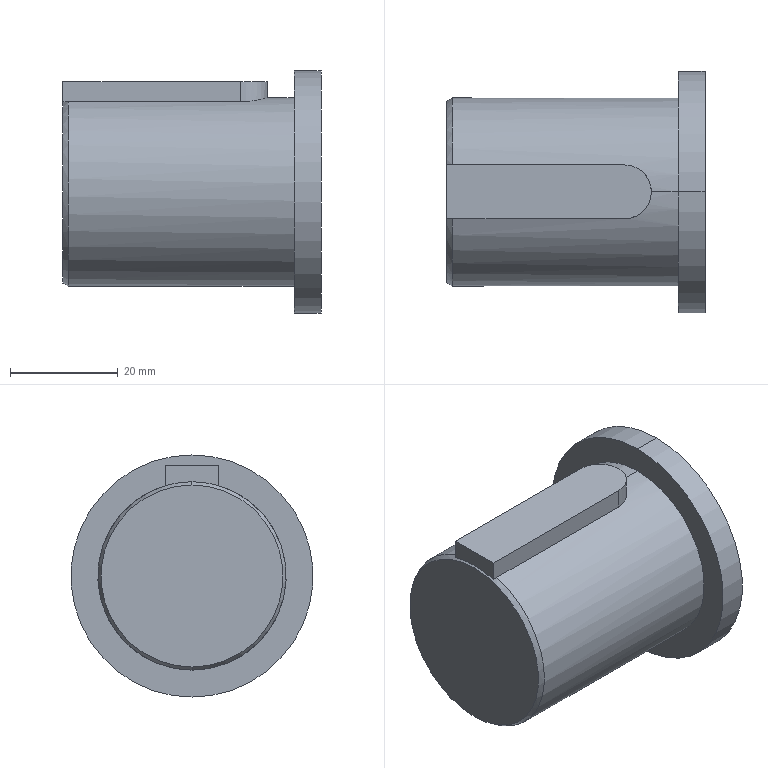Part | STEP file | 1 solid | 17 faces | box 48 x 45 x 45 mm | volume 50486 mm3 | cylinder 8 | plane 7 | cone 2 | commonest cylinder face diameters 35 x4 10 x2 45 x2
STEP:
#1=CARTESIAN_POINT('',(0.,0.,0.));
#2=DIRECTION('',(0.,0.,1.));
#3=DIRECTION('',(1.,0.,0.));
#4=AXIS2_PLACEMENT_3D('',#1,#2,#3);
#5=CARTESIAN_POINT('',(-134.,0.,-16.923));
#6=VERTEX_POINT('',#5);
#7=CARTESIAN_POINT('',(-133.,0.,-17.5));
#8=VERTEX_POINT('',#7);
#9=CARTESIAN_POINT('',(-133.5,0.,-17.211));
#10=DIRECTION('',(0.866,0.,-0.5));
#11=VECTOR('',#10,1.);
#12=LINE('',#9,#11);
#13=CARTESIAN_POINT('',(-133.5,0.,0.));
#14=DIRECTION('',(1.,0.,0.));
#15=DIRECTION('',(0.,0.,-1.));
#16=AXIS2_PLACEMENT_3D('',#13,#14,#15);
#17=CONICAL_SURFACE('',#16,17.211,0.5236);
#18=CARTESIAN_POINT('',(0.,0.));
#19=DIRECTION('',(0.,1.));
#20=VECTOR('',#19,1.);
#21=LINE('',#18,#20);
#22=(GEOMETRIC_REPRESENTATION_CONTEXT(2)PARAMETRIC_REPRESENTATION_CONTEXT()REPRESENTATION_CONTEXT('',''));
#23=DEFINITIONAL_REPRESENTATION('',(#21),#22);
#24=PCURVE('',#17,#23);
#25=CARTESIAN_POINT('',(-133.5,0.,0.));
#26=DIRECTION('',(1.,0.,0.));
#27=DIRECTION('',(0.,0.,-1.));
#28=AXIS2_PLACEMENT_3D('',#25,#26,#27);
#29=CONICAL_SURFACE('',#28,17.211,0.5236);
#30=CARTESIAN_POINT('',(6.283,0.));
#31=DIRECTION('',(0.,1.));
#32=VECTOR('',#31,1.);
#33=LINE('',#30,#32);
#34=(GEOMETRIC_REPRESENTATION_CONTEXT(2)PARAMETRIC_REPRESENTATION_CONTEXT()REPRESENTATION_CONTEXT('',''));
#35=DEFINITIONAL_REPRESENTATION('',(#33),#34);
#36=PCURVE('',#29,#35);
#37=SURFACE_CURVE('',#12,(#24,#36),.PCURVE_S1.);
#38=EDGE_CURVE('',#6,#8,#37,.T.);
#39=ORIENTED_EDGE('',*,*,#38,.F.);
#40=CARTESIAN_POINT('',(-134.,0.,16.923));
#41=VERTEX_POINT('',#40);
#42=CARTESIAN_POINT('',(-134.,0.,0.));
#43=DIRECTION('',(1.,0.,0.));
#44=DIRECTION('',(0.,0.,-1.));
#45=AXIS2_PLACEMENT_3D('',#42,#43,#44);
#46=CIRCLE('',#45,16.923);
#47=CARTESIAN_POINT('',(0.,-0.5));
#48=DIRECTION('',(1.,0.));
#49=VECTOR('',#48,1.);
#50=LINE('',#47,#49);
#51=(GEOMETRIC_REPRESENTATION_CONTEXT(2)PARAMETRIC_REPRESENTATION_CONTEXT()REPRESENTATION_CONTEXT('',''));
#52=DEFINITIONAL_REPRESENTATION('',(#50),#51);
#53=PCURVE('',#17,#52);
#54=CARTESIAN_POINT('',(-134.,0.,-8.461));
#55=DIRECTION('',(-1.,0.,0.));
#56=DIRECTION('',(0.,0.,1.));
#57=AXIS2_PLACEMENT_3D('',#54,#55,#56);
#58=PLANE('',#57);
#59=CARTESIAN_POINT('',(-8.461,0.));
#60=CARTESIAN_POINT('',(-8.461,29.311));
#61=CARTESIAN_POINT('',(16.923,14.655));
#62=CARTESIAN_POINT('',(42.307,0.));
#63=CARTESIAN_POINT('',(16.923,-14.655));
#64=CARTESIAN_POINT('',(-8.461,-29.311));
#65=CARTESIAN_POINT('',(-8.461,0.));
#66=(BOUNDED_CURVE()B_SPLINE_CURVE(2,(#59,#60,#61,#62,#63,#64,#65),.UNSPECIFIED.,.T.,.F.)B_SPLINE_CURVE_WITH_KNOTS((1,2,2,2,2,1),(-2.094,0.,2.094,4.189,6.283,8.378),.UNSPECIFIED.)CURVE()GEOMETRIC_REPRESENTATION_ITEM()RATIONAL_B_SPLINE_CURVE((1.,0.5,1.,0.5,1.,0.5,1.))REPRESENTATION_ITEM(''));
#67=(GEOMETRIC_REPRESENTATION_CONTEXT(2)PARAMETRIC_REPRESENTATION_CONTEXT()REPRESENTATION_CONTEXT('',''));
#68=DEFINITIONAL_REPRESENTATION('',(#66),#67);
#69=PCURVE('',#58,#68);
#70=SURFACE_CURVE('',#46,(#53,#69),.PCURVE_S1.);
#71=EDGE_CURVE('',#6,#41,#70,.T.);
#72=ORIENTED_EDGE('',*,*,#71,.T.);
#73=CARTESIAN_POINT('',(-133.,0.,17.5));
#74=VERTEX_POINT('',#73);
#75=CARTESIAN_POINT('',(-133.5,0.,17.211));
#76=DIRECTION('',(-0.866,0.,-0.5));
#77=VECTOR('',#76,1.);
#78=LINE('',#75,#77);
#79=CARTESIAN_POINT('',(3.142,0.));
#80=DIRECTION('',(0.,-1.));
#81=VECTOR('',#80,1.);
#82=LINE('',#79,#81);
#83=(GEOMETRIC_REPRESENTATION_CONTEXT(2)PARAMETRIC_REPRESENTATION_CONTEXT()REPRESENTATION_CONTEXT('',''));
#84=DEFINITIONAL_REPRESENTATION('',(#82),#83);
#85=PCURVE('',#17,#84);
#86=CARTESIAN_POINT('',(3.142,0.));
#87=DIRECTION('',(0.,-1.));
#88=VECTOR('',#87,1.);
#89=LINE('',#86,#88);
#90=(GEOMETRIC_REPRESENTATION_CONTEXT(2)PARAMETRIC_REPRESENTATION_CONTEXT()REPRESENTATION_CONTEXT('',''));
#91=DEFINITIONAL_REPRESENTATION('',(#89),#90);
#92=PCURVE('',#29,#91);
#93=SURFACE_CURVE('',#78,(#85,#92),.PCURVE_S1.);
#94=EDGE_CURVE('',#74,#41,#93,.T.);
#95=ORIENTED_EDGE('',*,*,#94,.F.);
#96=CARTESIAN_POINT('',(-133.,5.,16.771));
#97=VERTEX_POINT('',#96);
#98=CARTESIAN_POINT('',(-133.,0.,0.));
#99=DIRECTION('',(1.,0.,0.));
#100=DIRECTION('',(0.,0.,-1.));
#101=AXIS2_PLACEMENT_3D('',#98,#99,#100);
#102=CIRCLE('',#101,17.5);
#103=CARTESIAN_POINT('',(0.,0.5));
#104=DIRECTION('',(1.,0.));
#105=VECTOR('',#104,1.);
#106=LINE('',#103,#105);
#107=(GEOMETRIC_REPRESENTATION_CONTEXT(2)PARAMETRIC_REPRESENTATION_CONTEXT()REPRESENTATION_CONTEXT('',''));
#108=DEFINITIONAL_REPRESENTATION('',(#106),#107);
#109=PCURVE('',#17,#108);
#110=CARTESIAN_POINT('',(-133.5,0.,0.));
#111=DIRECTION('',(-1.,0.,0.));
#112=DIRECTION('',(0.,0.,-1.));
#113=AXIS2_PLACEMENT_3D('',#110,#111,#112);
#114=CYLINDRICAL_SURFACE('',#113,17.5);
#115=CARTESIAN_POINT('',(6.283,-0.5));
#116=DIRECTION('',(-1.,0.));
#117=VECTOR('',#116,1.);
#118=LINE('',#115,#117);
#119=(GEOMETRIC_REPRESENTATION_CONTEXT(2)PARAMETRIC_REPRESENTATION_CONTEXT()REPRESENTATION_CONTEXT('',''));
#120=DEFINITIONAL_REPRESENTATION('',(#118),#119);
#121=PCURVE('',#114,#120);
#122=SURFACE_CURVE('',#102,(#109,#121),.PCURVE_S1.);
#123=EDGE_CURVE('',#97,#74,#122,.T.);
#124=ORIENTED_EDGE('',*,*,#123,.F.);
#125=CARTESIAN_POINT('',(-133.,0.,0.));
#126=DIRECTION('',(1.,0.,0.));
#127=DIRECTION('',(0.,0.,-1.));
#128=AXIS2_PLACEMENT_3D('',#125,#126,#127);
#129=CIRCLE('',#128,17.5);
#130=CARTESIAN_POINT('',(0.,0.5));
#131=DIRECTION('',(1.,0.));
#132=VECTOR('',#131,1.);
#133=LINE('',#130,#132);
#134=(GEOMETRIC_REPRESENTATION_CONTEXT(2)PARAMETRIC_REPRESENTATION_CONTEXT()REPRESENTATION_CONTEXT('',''));
#135=DEFINITIONAL_REPRESENTATION('',(#133),#134);
#136=PCURVE('',#17,#135);
#137=CARTESIAN_POINT('',(-125.5,0.,0.));
#138=DIRECTION('',(-1.,0.,0.));
#139=DIRECTION('',(0.,0.,-1.));
#140=AXIS2_PLACEMENT_3D('',#137,#138,#139);
#141=CYLINDRICAL_SURFACE('',#140,17.5);
#142=CARTESIAN_POINT('',(6.283,7.5));
#143=DIRECTION('',(-1.,0.));
#144=VECTOR('',#143,1.);
#145=LINE('',#142,#144);
#146=(GEOMETRIC_REPRESENTATION_CONTEXT(2)PARAMETRIC_REPRESENTATION_CONTEXT()REPRESENTATION_CONTEXT('',''));
#147=DEFINITIONAL_REPRESENTATION('',(#145),#146);
#148=PCURVE('',#141,#147);
#149=SURFACE_CURVE('',#129,(#136,#148),.PCURVE_S1.);
#150=EDGE_CURVE('',#8,#97,#149,.T.);
#151=ORIENTED_EDGE('',*,*,#150,.F.);
#152=EDGE_LOOP('',(#39,#72,#95,#124,#151));
#153=FACE_BOUND('',#152,.T.);
#154=ADVANCED_FACE('',(#153),#17,.T.);
#155=ORIENTED_EDGE('',*,*,#123,.F.);
#156=CARTESIAN_POINT('',(-134.,5.,16.771));
#157=VERTEX_POINT('',#156);
#158=CARTESIAN_POINT('',(-133.5,5.,16.771));
#159=DIRECTION('',(1.,0.,0.));
#160=VECTOR('',#159,1.);
#161=LINE('',#158,#160);
#162=CARTESIAN_POINT('',(3.431,0.));
#163=DIRECTION('',(0.,-1.));
#164=VECTOR('',#163,1.);
#165=LINE('',#162,#164);
#166=(GEOMETRIC_REPRESENTATION_CONTEXT(2)PARAMETRIC_REPRESENTATION_CONTEXT()REPRESENTATION_CONTEXT('',''));
#167=DEFINITIONAL_REPRESENTATION('',(#165),#166);
#168=PCURVE('',#114,#167);
#169=CARTESIAN_POINT('',(-126.,5.,16.5));
#170=DIRECTION('',(0.,-1.,0.));
#171=DIRECTION('',(0.,0.,-1.));
#172=AXIS2_PLACEMENT_3D('',#169,#170,#171);
#173=PLANE('',#172);
#174=CARTESIAN_POINT('',(-0.2705,-7.5));
#175=DIRECTION('',(0.,1.));
#176=VECTOR('',#175,1.);
#177=LINE('',#174,#176);
#178=(GEOMETRIC_REPRESENTATION_CONTEXT(2)PARAMETRIC_REPRESENTATION_CONTEXT()REPRESENTATION_CONTEXT('',''));
#179=DEFINITIONAL_REPRESENTATION('',(#177),#178);
#180=PCURVE('',#173,#179);
#181=SURFACE_CURVE('',#161,(#168,#180),.PCURVE_S1.);
#182=EDGE_CURVE('',#157,#97,#181,.T.);
#183=ORIENTED_EDGE('',*,*,#182,.F.);
#184=CARTESIAN_POINT('',(-134.,0.,17.5));
#185=VERTEX_POINT('',#184);
#186=CARTESIAN_POINT('',(-134.,0.,0.));
#187=DIRECTION('',(-1.,0.,0.));
#188=DIRECTION('',(0.,0.,-1.));
#189=AXIS2_PLACEMENT_3D('',#186,#187,#188);
#190=CIRCLE('',#189,17.5);
#191=CARTESIAN_POINT('',(0.,0.5));
#192=DIRECTION('',(1.,0.));
#193=VECTOR('',#192,1.);
#194=LINE('',#191,#193);
#195=(GEOMETRIC_REPRESENTATION_CONTEXT(2)PARAMETRIC_REPRESENTATION_CONTEXT()REPRESENTATION_CONTEXT('',''));
#196=DEFINITIONAL_REPRESENTATION('',(#194),#195);
#197=PCURVE('',#114,#196);
#198=CARTESIAN_POINT('',(-134.,0.,0.));
#199=DIRECTION('',(1.,0.,0.));
#200=DIRECTION('',(0.,0.,-1.));
#201=AXIS2_PLACEMENT_3D('',#198,#199,#200);
#202=PLANE('',#201);
#203=CARTESIAN_POINT('',(17.5,0.));
#204=CARTESIAN_POINT('',(17.5,-30.311));
#205=CARTESIAN_POINT('',(-8.75,-15.155));
#206=CARTESIAN_POINT('',(-35.,0.));
#207=CARTESIAN_POINT('',(-8.75,15.155));
#208=CARTESIAN_POINT('',(17.5,30.311));
#209=CARTESIAN_POINT('',(17.5,0.));
#210=(BOUNDED_CURVE()B_SPLINE_CURVE(2,(#203,#204,#205,#206,#207,#208,#209),.UNSPECIFIED.,.T.,.F.)B_SPLINE_CURVE_WITH_KNOTS((1,2,2,2,2,1),(-2.094,0.,2.094,4.189,6.283,8.378),.UNSPECIFIED.)CURVE()GEOMETRIC_REPRESENTATION_ITEM()RATIONAL_B_SPLINE_CURVE((1.,0.5,1.,0.5,1.,0.5,1.))REPRESENTATION_ITEM(''));
#211=(GEOMETRIC_REPRESENTATION_CONTEXT(2)PARAMETRIC_REPRESENTATION_CONTEXT()REPRESENTATION_CONTEXT('',''));
#212=DEFINITIONAL_REPRESENTATION('',(#210),#211);
#213=PCURVE('',#202,#212);
#214=SURFACE_CURVE('',#190,(#197,#213),.PCURVE_S1.);
#215=EDGE_CURVE('',#185,#157,#214,.T.);
#216=ORIENTED_EDGE('',*,*,#215,.F.);
#217=CARTESIAN_POINT('',(-133.5,0.,17.5));
#218=DIRECTION('',(1.,0.,0.));
#219=VECTOR('',#218,1.);
#220=LINE('',#217,#219);
#221=CARTESIAN_POINT('',(3.142,0.));
#222=DIRECTION('',(0.,-1.));
#223=VECTOR('',#222,1.);
#224=LINE('',#221,#223);
#225=(GEOMETRIC_REPRESENTATION_CONTEXT(2)PARAMETRIC_REPRESENTATION_CONTEXT()REPRESENTATION_CONTEXT('',''));
#226=DEFINITIONAL_REPRESENTATION('',(#224),#225);
#227=PCURVE('',#114,#226);
#228=CARTESIAN_POINT('',(-133.5,0.,0.));
#229=DIRECTION('',(-1.,0.,0.));
#230=DIRECTION('',(0.,0.,-1.));
#231=AXIS2_PLACEMENT_3D('',#228,#229,#230);
#232=CYLINDRICAL_SURFACE('',#231,17.5);
#233=CARTESIAN_POINT('',(3.142,0.));
#234=DIRECTION('',(0.,-1.));
#235=VECTOR('',#234,1.);
#236=LINE('',#233,#235);
#237=(GEOMETRIC_REPRESENTATION_CONTEXT(2)PARAMETRIC_REPRESENTATION_CONTEXT()REPRESENTATION_CONTEXT('',''));
#238=DEFINITIONAL_REPRESENTATION('',(#236),#237);
#239=PCURVE('',#232,#238);
#240=SURFACE_CURVE('',#220,(#227,#239),.PCURVE_S1.);
#241=EDGE_CURVE('',#185,#74,#240,.T.);
#242=ORIENTED_EDGE('',*,*,#241,.T.);
#243=EDGE_LOOP('',(#155,#183,#216,#242));
#244=FACE_BOUND('',#243,.F.);
#245=ADVANCED_FACE('',(#244),#114,.F.);
#246=CARTESIAN_POINT('',(-134.,5.,20.5));
#247=VERTEX_POINT('',#246);
#248=CARTESIAN_POINT('',(-134.,-5.,20.5));
#249=VERTEX_POINT('',#248);
#250=CARTESIAN_POINT('',(-134.,0.,20.5));
#251=DIRECTION('',(0.,-1.,0.));
#252=VECTOR('',#251,1.);
#253=LINE('',#250,#252);
#254=CARTESIAN_POINT('',(-20.5,0.));
#255=DIRECTION('',(0.,-1.));
#256=VECTOR('',#255,1.);
#257=LINE('',#254,#256);
#258=(GEOMETRIC_REPRESENTATION_CONTEXT(2)PARAMETRIC_REPRESENTATION_CONTEXT()REPRESENTATION_CONTEXT('',''));
#259=DEFINITIONAL_REPRESENTATION('',(#257),#258);
#260=PCURVE('',#202,#259);
#261=CARTESIAN_POINT('',(-151.,0.,20.5));
#262=DIRECTION('',(0.,0.,1.));
#263=DIRECTION('',(1.,0.,0.));
#264=AXIS2_PLACEMENT_3D('',#261,#262,#263);
#265=PLANE('',#264);
#266=CARTESIAN_POINT('',(17.,0.));
#267=DIRECTION('',(0.,-1.));
#268=VECTOR('',#267,1.);
#269=LINE('',#266,#268);
#270=(GEOMETRIC_REPRESENTATION_CONTEXT(2)PARAMETRIC_REPRESENTATION_CONTEXT()REPRESENTATION_CONTEXT('',''));
#271=DEFINITIONAL_REPRESENTATION('',(#269),#270);
#272=PCURVE('',#265,#271);
#273=SURFACE_CURVE('',#253,(#260,#272),.PCURVE_S1.);
#274=EDGE_CURVE('',#247,#249,#273,.T.);
#275=ORIENTED_EDGE('',*,*,#274,.F.);
#276=CARTESIAN_POINT('',(-134.,5.,8.25));
#277=DIRECTION('',(0.,0.,1.));
#278=VECTOR('',#277,1.);
#279=LINE('',#276,#278);
#280=CARTESIAN_POINT('',(-8.25,5.));
#281=DIRECTION('',(-1.,0.));
#282=VECTOR('',#281,1.);
#283=LINE('',#280,#282);
#284=(GEOMETRIC_REPRESENTATION_CONTEXT(2)PARAMETRIC_REPRESENTATION_CONTEXT()REPRESENTATION_CONTEXT('',''));
#285=DEFINITIONAL_REPRESENTATION('',(#283),#284);
#286=PCURVE('',#202,#285);
#287=CARTESIAN_POINT('',(8.25,-8.));
#288=DIRECTION('',(-1.,0.));
#289=VECTOR('',#288,1.);
#290=LINE('',#287,#289);
#291=(GEOMETRIC_REPRESENTATION_CONTEXT(2)PARAMETRIC_REPRESENTATION_CONTEXT()REPRESENTATION_CONTEXT('',''));
#292=DEFINITIONAL_REPRESENTATION('',(#290),#291);
#293=PCURVE('',#173,#292);
#294=SURFACE_CURVE('',#279,(#286,#293),.PCURVE_S1.);
#295=EDGE_CURVE('',#157,#247,#294,.T.);
#296=ORIENTED_EDGE('',*,*,#295,.F.);
#297=ORIENTED_EDGE('',*,*,#215,.F.);
#298=CARTESIAN_POINT('',(-134.,-5.,16.771));
#299=VERTEX_POINT('',#298);
#300=CARTESIAN_POINT('',(-134.,0.,0.));
#301=DIRECTION('',(-1.,0.,0.));
#302=DIRECTION('',(0.,0.,-1.));
#303=AXIS2_PLACEMENT_3D('',#300,#301,#302);
#304=CIRCLE('',#303,17.5);
#305=CARTESIAN_POINT('',(17.5,0.));
#306=CARTESIAN_POINT('',(17.5,-30.311));
#307=CARTESIAN_POINT('',(-8.75,-15.155));
#308=CARTESIAN_POINT('',(-35.,0.));
#309=CARTESIAN_POINT('',(-8.75,15.155));
#310=CARTESIAN_POINT('',(17.5,30.311));
#311=CARTESIAN_POINT('',(17.5,0.));
#312=(BOUNDED_CURVE()B_SPLINE_CURVE(2,(#305,#306,#307,#308,#309,#310,#311),.UNSPECIFIED.,.T.,.F.)B_SPLINE_CURVE_WITH_KNOTS((1,2,2,2,2,1),(-2.094,0.,2.094,4.189,6.283,8.378),.UNSPECIFIED.)CURVE()GEOMETRIC_REPRESENTATION_ITEM()RATIONAL_B_SPLINE_CURVE((1.,0.5,1.,0.5,1.,0.5,1.))REPRESENTATION_ITEM(''));
#313=(GEOMETRIC_REPRESENTATION_CONTEXT(2)PARAMETRIC_REPRESENTATION_CONTEXT()REPRESENTATION_CONTEXT('',''));
#314=DEFINITIONAL_REPRESENTATION('',(#312),#313);
#315=PCURVE('',#202,#314);
#316=CARTESIAN_POINT('',(0.,0.5));
#317=DIRECTION('',(1.,0.));
#318=VECTOR('',#317,1.);
#319=LINE('',#316,#318);
#320=(GEOMETRIC_REPRESENTATION_CONTEXT(2)PARAMETRIC_REPRESENTATION_CONTEXT()REPRESENTATION_CONTEXT('',''));
#321=DEFINITIONAL_REPRESENTATION('',(#319),#320);
#322=PCURVE('',#232,#321);
#323=SURFACE_CURVE('',#304,(#315,#322),.PCURVE_S1.);
#324=EDGE_CURVE('',#299,#185,#323,.T.);
#325=ORIENTED_EDGE('',*,*,#324,.F.);
#326=CARTESIAN_POINT('',(-134.,-5.,8.25));
#327=DIRECTION('',(0.,0.,-1.));
#328=VECTOR('',#327,1.);
#329=LINE('',#326,#328);
#330=CARTESIAN_POINT('',(-8.25,-5.));
#331=DIRECTION('',(1.,0.));
#332=VECTOR('',#331,1.);
#333=LINE('',#330,#332);
#334=(GEOMETRIC_REPRESENTATION_CONTEXT(2)PARAMETRIC_REPRESENTATION_CONTEXT()REPRESENTATION_CONTEXT('',''));
#335=DEFINITIONAL_REPRESENTATION('',(#333),#334);
#336=PCURVE('',#202,#335);
#337=CARTESIAN_POINT('',(-126.,-5.,16.5));
#338=DIRECTION('',(0.,1.,0.));
#339=DIRECTION('',(1.,0.,0.));
#340=AXIS2_PLACEMENT_3D('',#337,#338,#339);
#341=PLANE('',#340);
#342=CARTESIAN_POINT('',(-8.,8.25));
#343=DIRECTION('',(0.,1.));
#344=VECTOR('',#343,1.);
#345=LINE('',#342,#344);
#346=(GEOMETRIC_REPRESENTATION_CONTEXT(2)PARAMETRIC_REPRESENTATION_CONTEXT()REPRESENTATION_CONTEXT('',''));
#347=DEFINITIONAL_REPRESENTATION('',(#345),#346);
#348=PCURVE('',#341,#347);
#349=SURFACE_CURVE('',#329,(#336,#348),.PCURVE_S1.);
#350=EDGE_CURVE('',#249,#299,#349,.T.);
#351=ORIENTED_EDGE('',*,*,#350,.F.);
#352=EDGE_LOOP('',(#275,#296,#297,#325,#351));
#353=FACE_BOUND('',#352,.T.);
#354=ADVANCED_FACE('',(#353),#202,.F.);
#355=ORIENTED_EDGE('',*,*,#324,.F.);
#356=CARTESIAN_POINT('',(-133.,-5.,16.771));
#357=VERTEX_POINT('',#356);
#358=CARTESIAN_POINT('',(-133.5,-5.,16.771));
#359=DIRECTION('',(-1.,0.,0.));
#360=VECTOR('',#359,1.);
#361=LINE('',#358,#360);
#362=CARTESIAN_POINT('',(2.852,0.));
#363=DIRECTION('',(0.,1.));
#364=VECTOR('',#363,1.);
#365=LINE('',#362,#364);
#366=(GEOMETRIC_REPRESENTATION_CONTEXT(2)PARAMETRIC_REPRESENTATION_CONTEXT()REPRESENTATION_CONTEXT('',''));
#367=DEFINITIONAL_REPRESENTATION('',(#365),#366);
#368=PCURVE('',#232,#367);
#369=CARTESIAN_POINT('',(-7.5,-0.2705));
#370=DIRECTION('',(-1.,0.));
#371=VECTOR('',#370,1.);
#372=LINE('',#369,#371);
#373=(GEOMETRIC_REPRESENTATION_CONTEXT(2)PARAMETRIC_REPRESENTATION_CONTEXT()REPRESENTATION_CONTEXT('',''));
#374=DEFINITIONAL_REPRESENTATION('',(#372),#373);
#375=PCURVE('',#341,#374);
#376=SURFACE_CURVE('',#361,(#368,#375),.PCURVE_S1.);
#377=EDGE_CURVE('',#357,#299,#376,.T.);
#378=ORIENTED_EDGE('',*,*,#377,.F.);
#379=CARTESIAN_POINT('',(-133.,0.,0.));
#380=DIRECTION('',(1.,0.,0.));
#381=DIRECTION('',(0.,0.,-1.));
#382=AXIS2_PLACEMENT_3D('',#379,#380,#381);
#383=CIRCLE('',#382,17.5);
#384=CARTESIAN_POINT('',(6.283,-0.5));
#385=DIRECTION('',(-1.,0.));
#386=VECTOR('',#385,1.);
#387=LINE('',#384,#386);
#388=(GEOMETRIC_REPRESENTATION_CONTEXT(2)PARAMETRIC_REPRESENTATION_CONTEXT()REPRESENTATION_CONTEXT('',''));
#389=DEFINITIONAL_REPRESENTATION('',(#387),#388);
#390=PCURVE('',#232,#389);
#391=CARTESIAN_POINT('',(0.,0.5));
#392=DIRECTION('',(1.,0.));
#393=VECTOR('',#392,1.);
#394=LINE('',#391,#393);
#395=(GEOMETRIC_REPRESENTATION_CONTEXT(2)PARAMETRIC_REPRESENTATION_CONTEXT()REPRESENTATION_CONTEXT('',''));
#396=DEFINITIONAL_REPRESENTATION('',(#394),#395);
#397=PCURVE('',#29,#396);
#398=SURFACE_CURVE('',#383,(#390,#397),.PCURVE_S1.);
#399=EDGE_CURVE('',#74,#357,#398,.T.);
#400=ORIENTED_EDGE('',*,*,#399,.F.);
#401=ORIENTED_EDGE('',*,*,#241,.F.);
#402=EDGE_LOOP('',(#355,#378,#400,#401));
#403=FACE_BOUND('',#402,.F.);
#404=ADVANCED_FACE('',(#403),#232,.F.);
#405=ORIENTED_EDGE('',*,*,#295,.T.);
#406=CARTESIAN_POINT('',(-101.,5.,20.5));
#407=VERTEX_POINT('',#406);
#408=CARTESIAN_POINT('',(-126.,5.,20.5));
#409=DIRECTION('',(-1.,0.,0.));
#410=VECTOR('',#409,1.);
#411=LINE('',#408,#410);
#412=CARTESIAN_POINT('',(-4.,0.));
#413=DIRECTION('',(0.,-1.));
#414=VECTOR('',#413,1.);
#415=LINE('',#412,#414);
#416=(GEOMETRIC_REPRESENTATION_CONTEXT(2)PARAMETRIC_REPRESENTATION_CONTEXT()REPRESENTATION_CONTEXT('',''));
#417=DEFINITIONAL_REPRESENTATION('',(#415),#416);
#418=PCURVE('',#173,#417);
#419=CARTESIAN_POINT('',(25.,5.));
#420=DIRECTION('',(-1.,0.));
#421=VECTOR('',#420,1.);
#422=LINE('',#419,#421);
#423=(GEOMETRIC_REPRESENTATION_CONTEXT(2)PARAMETRIC_REPRESENTATION_CONTEXT()REPRESENTATION_CONTEXT('',''));
#424=DEFINITIONAL_REPRESENTATION('',(#422),#423);
#425=PCURVE('',#265,#424);
#426=SURFACE_CURVE('',#411,(#418,#425),.PCURVE_S1.);
#427=EDGE_CURVE('',#407,#247,#426,.T.);
#428=ORIENTED_EDGE('',*,*,#427,.F.);
#429=CARTESIAN_POINT('',(-101.,5.,16.771));
#430=VERTEX_POINT('',#429);
#431=CARTESIAN_POINT('',(-101.,5.,16.5));
#432=DIRECTION('',(0.,0.,-1.));
#433=VECTOR('',#432,1.);
#434=LINE('',#431,#433);
#435=CARTESIAN_POINT('',(0.,25.));
#436=DIRECTION('',(1.,0.));
#437=VECTOR('',#436,1.);
#438=LINE('',#435,#437);
#439=(GEOMETRIC_REPRESENTATION_CONTEXT(2)PARAMETRIC_REPRESENTATION_CONTEXT()REPRESENTATION_CONTEXT('',''));
#440=DEFINITIONAL_REPRESENTATION('',(#438),#439);
#441=PCURVE('',#173,#440);
#442=CARTESIAN_POINT('',(-101.,0.,16.5));
#443=DIRECTION('',(0.,0.,1.));
#444=DIRECTION('',(1.,0.,0.));
#445=AXIS2_PLACEMENT_3D('',#442,#443,#444);
#446=CYLINDRICAL_SURFACE('',#445,5.);
#447=CARTESIAN_POINT('',(1.571,0.));
#448=DIRECTION('',(0.,-1.));
#449=VECTOR('',#448,1.);
#450=LINE('',#447,#449);
#451=(GEOMETRIC_REPRESENTATION_CONTEXT(2)PARAMETRIC_REPRESENTATION_CONTEXT()REPRESENTATION_CONTEXT('',''));
#452=DEFINITIONAL_REPRESENTATION('',(#450),#451);
#453=PCURVE('',#446,#452);
#454=SURFACE_CURVE('',#434,(#441,#453),.PCURVE_S1.);
#455=EDGE_CURVE('',#407,#430,#454,.T.);
#456=ORIENTED_EDGE('',*,*,#455,.T.);
#457=CARTESIAN_POINT('',(-125.5,5.,16.771));
#458=DIRECTION('',(1.,0.,0.));
#459=VECTOR('',#458,1.);
#460=LINE('',#457,#459);
#461=CARTESIAN_POINT('',(-0.2705,0.5));
#462=DIRECTION('',(0.,1.));
#463=VECTOR('',#462,1.);
#464=LINE('',#461,#463);
#465=(GEOMETRIC_REPRESENTATION_CONTEXT(2)PARAMETRIC_REPRESENTATION_CONTEXT()REPRESENTATION_CONTEXT('',''));
#466=DEFINITIONAL_REPRESENTATION('',(#464),#465);
#467=PCURVE('',#173,#466);
#468=CARTESIAN_POINT('',(3.431,0.));
#469=DIRECTION('',(0.,-1.));
#470=VECTOR('',#469,1.);
#471=LINE('',#468,#470);
#472=(GEOMETRIC_REPRESENTATION_CONTEXT(2)PARAMETRIC_REPRESENTATION_CONTEXT()REPRESENTATION_CONTEXT('',''));
#473=DEFINITIONAL_REPRESENTATION('',(#471),#472);
#474=PCURVE('',#141,#473);
#475=SURFACE_CURVE('',#460,(#467,#474),.PCURVE_S1.);
#476=EDGE_CURVE('',#97,#430,#475,.T.);
#477=ORIENTED_EDGE('',*,*,#476,.F.);
#478=ORIENTED_EDGE('',*,*,#182,.F.);
#479=EDGE_LOOP('',(#405,#428,#456,#477,#478));
#480=FACE_BOUND('',#479,.T.);
#481=ADVANCED_FACE('',(#480),#173,.F.);
#482=ORIENTED_EDGE('',*,*,#38,.T.);
#483=CARTESIAN_POINT('',(-133.,0.,0.));
#484=DIRECTION('',(1.,0.,0.));
#485=DIRECTION('',(0.,0.,-1.));
#486=AXIS2_PLACEMENT_3D('',#483,#484,#485);
#487=CIRCLE('',#486,17.5);
#488=CARTESIAN_POINT('',(0.,0.5));
#489=DIRECTION('',(1.,0.));
#490=VECTOR('',#489,1.);
#491=LINE('',#488,#490);
#492=(GEOMETRIC_REPRESENTATION_CONTEXT(2)PARAMETRIC_REPRESENTATION_CONTEXT()REPRESENTATION_CONTEXT('',''));
#493=DEFINITIONAL_REPRESENTATION('',(#491),#492);
#494=PCURVE('',#29,#493);
#495=CARTESIAN_POINT('',(-125.5,0.,0.));
#496=DIRECTION('',(-1.,0.,0.));
#497=DIRECTION('',(0.,0.,-1.));
#498=AXIS2_PLACEMENT_3D('',#495,#496,#497);
#499=CYLINDRICAL_SURFACE('',#498,17.5);
#500=CARTESIAN_POINT('',(6.283,7.5));
#501=DIRECTION('',(-1.,0.));
#502=VECTOR('',#501,1.);
#503=LINE('',#500,#502);
#504=(GEOMETRIC_REPRESENTATION_CONTEXT(2)PARAMETRIC_REPRESENTATION_CONTEXT()REPRESENTATION_CONTEXT('',''));
#505=DEFINITIONAL_REPRESENTATION('',(#503),#504);
#506=PCURVE('',#499,#505);
#507=SURFACE_CURVE('',#487,(#494,#506),.PCURVE_S1.);
#508=EDGE_CURVE('',#357,#8,#507,.T.);
#509=ORIENTED_EDGE('',*,*,#508,.F.);
#510=ORIENTED_EDGE('',*,*,#399,.F.);
#511=ORIENTED_EDGE('',*,*,#94,.T.);
#512=CARTESIAN_POINT('',(-134.,0.,0.));
#513=DIRECTION('',(1.,0.,0.));
#514=DIRECTION('',(0.,0.,-1.));
#515=AXIS2_PLACEMENT_3D('',#512,#513,#514);
#516=CIRCLE('',#515,16.923);
#517=CARTESIAN_POINT('',(0.,-0.5));
#518=DIRECTION('',(1.,0.));
#519=VECTOR('',#518,1.);
#520=LINE('',#517,#519);
#521=(GEOMETRIC_REPRESENTATION_CONTEXT(2)PARAMETRIC_REPRESENTATION_CONTEXT()REPRESENTATION_CONTEXT('',''));
#522=DEFINITIONAL_REPRESENTATION('',(#520),#521);
#523=PCURVE('',#29,#522);
#524=CARTESIAN_POINT('',(-8.461,0.));
#525=CARTESIAN_POINT('',(-8.461,29.311));
#526=CARTESIAN_POINT('',(16.923,14.655));
#527=CARTESIAN_POINT('',(42.307,0.));
#528=CARTESIAN_POINT('',(16.923,-14.655));
#529=CARTESIAN_POINT('',(-8.461,-29.311));
#530=CARTESIAN_POINT('',(-8.461,0.));
#531=(BOUNDED_CURVE()B_SPLINE_CURVE(2,(#524,#525,#526,#527,#528,#529,#530),.UNSPECIFIED.,.T.,.F.)B_SPLINE_CURVE_WITH_KNOTS((1,2,2,2,2,1),(-2.094,0.,2.094,4.189,6.283,8.378),.UNSPECIFIED.)CURVE()GEOMETRIC_REPRESENTATION_ITEM()RATIONAL_B_SPLINE_CURVE((1.,0.5,1.,0.5,1.,0.5,1.))REPRESENTATION_ITEM(''));
#532=(GEOMETRIC_REPRESENTATION_CONTEXT(2)PARAMETRIC_REPRESENTATION_CONTEXT()REPRESENTATION_CONTEXT('',''));
#533=DEFINITIONAL_REPRESENTATION('',(#531),#532);
#534=PCURVE('',#58,#533);
#535=SURFACE_CURVE('',#516,(#523,#534),.PCURVE_S1.);
#536=EDGE_CURVE('',#41,#6,#535,.T.);
#537=ORIENTED_EDGE('',*,*,#536,.T.);
#538=EDGE_LOOP('',(#482,#509,#510,#511,#537));
#539=FACE_BOUND('',#538,.T.);
#540=ADVANCED_FACE('',(#539),#29,.T.);
#541=ORIENTED_EDGE('',*,*,#274,.T.);
#542=CARTESIAN_POINT('',(-101.,-5.,20.5));
#543=VERTEX_POINT('',#542);
#544=CARTESIAN_POINT('',(-126.,-5.,20.5));
#545=DIRECTION('',(1.,0.,0.));
#546=VECTOR('',#545,1.);
#547=LINE('',#544,#546);
#548=CARTESIAN_POINT('',(25.,-5.));
#549=DIRECTION('',(1.,0.));
#550=VECTOR('',#549,1.);
#551=LINE('',#548,#550);
#552=(GEOMETRIC_REPRESENTATION_CONTEXT(2)PARAMETRIC_REPRESENTATION_CONTEXT()REPRESENTATION_CONTEXT('',''));
#553=DEFINITIONAL_REPRESENTATION('',(#551),#552);
#554=PCURVE('',#265,#553);
#555=CARTESIAN_POINT('',(0.,-4.));
#556=DIRECTION('',(1.,0.));
#557=VECTOR('',#556,1.);
#558=LINE('',#555,#557);
#559=(GEOMETRIC_REPRESENTATION_CONTEXT(2)PARAMETRIC_REPRESENTATION_CONTEXT()REPRESENTATION_CONTEXT('',''));
#560=DEFINITIONAL_REPRESENTATION('',(#558),#559);
#561=PCURVE('',#341,#560);
#562=SURFACE_CURVE('',#547,(#554,#561),.PCURVE_S1.);
#563=EDGE_CURVE('',#249,#543,#562,.T.);
#564=ORIENTED_EDGE('',*,*,#563,.T.);
#565=CARTESIAN_POINT('',(-96.,0.,20.5));
#566=VERTEX_POINT('',#565);
#567=CARTESIAN_POINT('',(-101.,0.,20.5));
#568=DIRECTION('',(0.,0.,1.));
#569=DIRECTION('',(1.,0.,0.));
#570=AXIS2_PLACEMENT_3D('',#567,#568,#569);
#571=CIRCLE('',#570,5.);
#572=CARTESIAN_POINT('',(50.,0.));
#573=DIRECTION('',(1.,0.));
#574=AXIS2_PLACEMENT_2D('',#572,#573);
#575=CIRCLE('',#574,5.);
#576=(GEOMETRIC_REPRESENTATION_CONTEXT(2)PARAMETRIC_REPRESENTATION_CONTEXT()REPRESENTATION_CONTEXT('',''));
#577=DEFINITIONAL_REPRESENTATION('',(#575),#576);
#578=PCURVE('',#265,#577);
#579=CARTESIAN_POINT('',(-101.,0.,16.5));
#580=DIRECTION('',(0.,0.,1.));
#581=DIRECTION('',(1.,0.,0.));
#582=AXIS2_PLACEMENT_3D('',#579,#580,#581);
#583=CYLINDRICAL_SURFACE('',#582,5.);
#584=CARTESIAN_POINT('',(0.,4.));
#585=DIRECTION('',(1.,0.));
#586=VECTOR('',#585,1.);
#587=LINE('',#584,#586);
#588=(GEOMETRIC_REPRESENTATION_CONTEXT(2)PARAMETRIC_REPRESENTATION_CONTEXT()REPRESENTATION_CONTEXT('',''));
#589=DEFINITIONAL_REPRESENTATION('',(#587),#588);
#590=PCURVE('',#583,#589);
#591=SURFACE_CURVE('',#571,(#578,#590),.PCURVE_S1.);
#592=EDGE_CURVE('',#543,#566,#591,.T.);
#593=ORIENTED_EDGE('',*,*,#592,.T.);
#594=CARTESIAN_POINT('',(-101.,0.,20.5));
#595=DIRECTION('',(0.,0.,1.));
#596=DIRECTION('',(1.,0.,0.));
#597=AXIS2_PLACEMENT_3D('',#594,#595,#596);
#598=CIRCLE('',#597,5.);
#599=CARTESIAN_POINT('',(50.,0.));
#600=DIRECTION('',(1.,0.));
#601=AXIS2_PLACEMENT_2D('',#599,#600);
#602=CIRCLE('',#601,5.);
#603=(GEOMETRIC_REPRESENTATION_CONTEXT(2)PARAMETRIC_REPRESENTATION_CONTEXT()REPRESENTATION_CONTEXT('',''));
#604=DEFINITIONAL_REPRESENTATION('',(#602),#603);
#605=PCURVE('',#265,#604);
#606=CARTESIAN_POINT('',(0.,4.));
#607=DIRECTION('',(1.,0.));
#608=VECTOR('',#607,1.);
#609=LINE('',#606,#608);
#610=(GEOMETRIC_REPRESENTATION_CONTEXT(2)PARAMETRIC_REPRESENTATION_CONTEXT()REPRESENTATION_CONTEXT('',''));
#611=DEFINITIONAL_REPRESENTATION('',(#609),#610);
#612=PCURVE('',#446,#611);
#613=SURFACE_CURVE('',#598,(#605,#612),.PCURVE_S1.);
#614=EDGE_CURVE('',#566,#407,#613,.T.);
#615=ORIENTED_EDGE('',*,*,#614,.T.);
#616=ORIENTED_EDGE('',*,*,#427,.T.);
#617=EDGE_LOOP('',(#541,#564,#593,#615,#616));
#618=FACE_BOUND('',#617,.T.);
#619=ADVANCED_FACE('',(#618),#265,.T.);
#620=ORIENTED_EDGE('',*,*,#536,.F.);
#621=ORIENTED_EDGE('',*,*,#71,.F.);
#622=EDGE_LOOP('',(#620,#621));
#623=FACE_BOUND('',#622,.T.);
#624=ADVANCED_FACE('',(#623),#58,.T.);
#625=ORIENTED_EDGE('',*,*,#350,.T.);
#626=ORIENTED_EDGE('',*,*,#377,.F.);
#627=CARTESIAN_POINT('',(-101.,-5.,16.771));
#628=VERTEX_POINT('',#627);
#629=CARTESIAN_POINT('',(-125.5,-5.,16.771));
#630=DIRECTION('',(-1.,0.,0.));
#631=VECTOR('',#630,1.);
#632=LINE('',#629,#631);
#633=CARTESIAN_POINT('',(0.5,-0.2705));
#634=DIRECTION('',(-1.,0.));
#635=VECTOR('',#634,1.);
#636=LINE('',#633,#635);
#637=(GEOMETRIC_REPRESENTATION_CONTEXT(2)PARAMETRIC_REPRESENTATION_CONTEXT()REPRESENTATION_CONTEXT('',''));
#638=DEFINITIONAL_REPRESENTATION('',(#636),#637);
#639=PCURVE('',#341,#638);
#640=CARTESIAN_POINT('',(2.852,0.));
#641=DIRECTION('',(0.,1.));
#642=VECTOR('',#641,1.);
#643=LINE('',#640,#642);
#644=(GEOMETRIC_REPRESENTATION_CONTEXT(2)PARAMETRIC_REPRESENTATION_CONTEXT()REPRESENTATION_CONTEXT('',''));
#645=DEFINITIONAL_REPRESENTATION('',(#643),#644);
#646=PCURVE('',#499,#645);
#647=SURFACE_CURVE('',#632,(#639,#646),.PCURVE_S1.);
#648=EDGE_CURVE('',#628,#357,#647,.T.);
#649=ORIENTED_EDGE('',*,*,#648,.F.);
#650=CARTESIAN_POINT('',(-101.,-5.,16.5));
#651=DIRECTION('',(0.,0.,-1.));
#652=VECTOR('',#651,1.);
#653=LINE('',#650,#652);
#654=CARTESIAN_POINT('',(25.,0.));
#655=DIRECTION('',(0.,1.));
#656=VECTOR('',#655,1.);
#657=LINE('',#654,#656);
#658=(GEOMETRIC_REPRESENTATION_CONTEXT(2)PARAMETRIC_REPRESENTATION_CONTEXT()REPRESENTATION_CONTEXT('',''));
#659=DEFINITIONAL_REPRESENTATION('',(#657),#658);
#660=PCURVE('',#341,#659);
#661=CARTESIAN_POINT('',(4.712,0.));
#662=DIRECTION('',(0.,-1.));
#663=VECTOR('',#662,1.);
#664=LINE('',#661,#663);
#665=(GEOMETRIC_REPRESENTATION_CONTEXT(2)PARAMETRIC_REPRESENTATION_CONTEXT()REPRESENTATION_CONTEXT('',''));
#666=DEFINITIONAL_REPRESENTATION('',(#664),#665);
#667=PCURVE('',#583,#666);
#668=SURFACE_CURVE('',#653,(#660,#667),.PCURVE_S1.);
#669=EDGE_CURVE('',#543,#628,#668,.T.);
#670=ORIENTED_EDGE('',*,*,#669,.F.);
#671=ORIENTED_EDGE('',*,*,#563,.F.);
#672=EDGE_LOOP('',(#625,#626,#649,#670,#671));
#673=FACE_BOUND('',#672,.T.);
#674=ADVANCED_FACE('',(#673),#341,.F.);
#675=CARTESIAN_POINT('',(-96.,0.,17.5));
#676=VERTEX_POINT('',#675);
#677=CARTESIAN_POINT('',(-96.,0.,16.5));
#678=DIRECTION('',(0.,0.,-1.));
#679=VECTOR('',#678,1.);
#680=LINE('',#677,#679);
#681=CARTESIAN_POINT('',(6.283,0.));
#682=DIRECTION('',(0.,-1.));
#683=VECTOR('',#682,1.);
#684=LINE('',#681,#683);
#685=(GEOMETRIC_REPRESENTATION_CONTEXT(2)PARAMETRIC_REPRESENTATION_CONTEXT()REPRESENTATION_CONTEXT('',''));
#686=DEFINITIONAL_REPRESENTATION('',(#684),#685);
#687=PCURVE('',#583,#686);
#688=CARTESIAN_POINT('',(0.,0.));
#689=DIRECTION('',(0.,-1.));
#690=VECTOR('',#689,1.);
#691=LINE('',#688,#690);
#692=(GEOMETRIC_REPRESENTATION_CONTEXT(2)PARAMETRIC_REPRESENTATION_CONTEXT()REPRESENTATION_CONTEXT('',''));
#693=DEFINITIONAL_REPRESENTATION('',(#691),#692);
#694=PCURVE('',#446,#693);
#695=SURFACE_CURVE('',#680,(#687,#694),.PCURVE_S1.);
#696=EDGE_CURVE('',#566,#676,#695,.T.);
#697=ORIENTED_EDGE('',*,*,#696,.F.);
#698=ORIENTED_EDGE('',*,*,#592,.F.);
#699=ORIENTED_EDGE('',*,*,#669,.T.);
#700=CARTESIAN_POINT('',(-96.,0.,17.5));
#701=CARTESIAN_POINT('',(-96.,-0.3158,17.5));
#702=CARTESIAN_POINT('',(-96.03,-0.6418,17.491));
#703=CARTESIAN_POINT('',(-96.158,-1.289,17.455));
#704=CARTESIAN_POINT('',(-96.255,-1.611,17.428));
#705=CARTESIAN_POINT('',(-96.51,-2.226,17.361));
#706=CARTESIAN_POINT('',(-96.669,-2.521,17.32));
#707=CARTESIAN_POINT('',(-97.036,-3.065,17.232));
#708=CARTESIAN_POINT('',(-97.244,-3.315,17.185));
#709=CARTESIAN_POINT('',(-97.685,-3.757,17.094));
#710=CARTESIAN_POINT('',(-97.935,-3.964,17.046));
#711=CARTESIAN_POINT('',(-98.479,-4.331,16.957));
#712=CARTESIAN_POINT('',(-98.774,-4.49,16.915));
#713=CARTESIAN_POINT('',(-99.389,-4.745,16.845));
#714=CARTESIAN_POINT('',(-99.711,-4.842,16.817));
#715=CARTESIAN_POINT('',(-100.358,-4.97,16.78));
#716=CARTESIAN_POINT('',(-100.684,-5.,16.771));
#717=CARTESIAN_POINT('',(-101.,-5.,16.771));
#718=B_SPLINE_CURVE_WITH_KNOTS('',3,(#700,#701,#702,#703,#704,#705,#706,#707,#708,#709,#710,#711,#712,#713,#714,#715,#716,#717),.UNSPECIFIED.,.F.,.F.,(4,2,2,2,2,2,2,2,4),(7.58,8.527,9.474,10.421,11.369,12.316,13.264,14.211,15.159),.UNSPECIFIED.);
#719=CARTESIAN_POINT('',(6.283,1.));
#720=CARTESIAN_POINT('',(6.272,1.));
#721=CARTESIAN_POINT('',(6.249,0.9994));
#722=CARTESIAN_POINT('',(6.214,0.9968));
#723=CARTESIAN_POINT('',(6.178,0.9924));
#724=CARTESIAN_POINT('',(6.143,0.9862));
#725=CARTESIAN_POINT('',(6.107,0.9783));
#726=CARTESIAN_POINT('',(6.071,0.9685));
#727=CARTESIAN_POINT('',(6.035,0.957));
#728=CARTESIAN_POINT('',(5.998,0.9438));
#729=CARTESIAN_POINT('',(5.962,0.9289));
#730=CARTESIAN_POINT('',(5.926,0.9126));
#731=CARTESIAN_POINT('',(5.889,0.8947));
#732=CARTESIAN_POINT('',(5.853,0.8755));
#733=CARTESIAN_POINT('',(5.817,0.8551));
#734=CARTESIAN_POINT('',(5.78,0.8336));
#735=CARTESIAN_POINT('',(5.744,0.811));
#736=CARTESIAN_POINT('',(5.708,0.7877));
#737=CARTESIAN_POINT('',(5.673,0.7637));
#738=CARTESIAN_POINT('',(5.637,0.7391));
#739=CARTESIAN_POINT('',(5.602,0.7143));
#740=CARTESIAN_POINT('',(5.567,0.6892));
#741=CARTESIAN_POINT('',(5.532,0.664));
#742=CARTESIAN_POINT('',(5.498,0.6391));
#743=CARTESIAN_POINT('',(5.463,0.6141));
#744=CARTESIAN_POINT('',(5.429,0.5888));
#745=CARTESIAN_POINT('',(5.394,0.5636));
#746=CARTESIAN_POINT('',(5.358,0.5384));
#747=CARTESIAN_POINT('',(5.323,0.5136));
#748=CARTESIAN_POINT('',(5.287,0.4892));
#749=CARTESIAN_POINT('',(5.251,0.4654));
#750=CARTESIAN_POINT('',(5.215,0.4424));
#751=CARTESIAN_POINT('',(5.179,0.4204));
#752=CARTESIAN_POINT('',(5.142,0.3994));
#753=CARTESIAN_POINT('',(5.106,0.3796));
#754=CARTESIAN_POINT('',(5.07,0.3612));
#755=CARTESIAN_POINT('',(5.033,0.3443));
#756=CARTESIAN_POINT('',(4.997,0.329));
#757=CARTESIAN_POINT('',(4.961,0.3153));
#758=CARTESIAN_POINT('',(4.925,0.3033));
#759=CARTESIAN_POINT('',(4.889,0.2931));
#760=CARTESIAN_POINT('',(4.853,0.2848));
#761=CARTESIAN_POINT('',(4.817,0.2784));
#762=CARTESIAN_POINT('',(4.782,0.2739));
#763=CARTESIAN_POINT('',(4.747,0.2711));
#764=CARTESIAN_POINT('',(4.724,0.2705));
#765=CARTESIAN_POINT('',(4.712,0.2705));
#766=B_SPLINE_CURVE_WITH_KNOTS('',3,(#719,#720,#721,#722,#723,#724,#725,#726,#727,#728,#729,#730,#731,#732,#733,#734,#735,#736,#737,#738,#739,#740,#741,#742,#743,#744,#745,#746,#747,#748,#749,#750,#751,#752,#753,#754,#755,#756,#757,#758,#759,#760,#761,#762,#763,#764,#765),.UNSPECIFIED.,.F.,.F.,(4,1,1,1,1,1,1,1,1,1,1,1,1,1,1,1,1,1,1,1,1,1,1,1,1,1,1,1,1,1,1,1,1,1,1,1,1,1,1,1,1,1,1,1,4),(7.58,7.752,7.924,8.096,8.269,8.441,8.613,8.785,8.958,9.13,9.302,9.474,9.647,9.819,9.991,10.163,10.336,10.508,10.68,10.852,11.025,11.197,11.369,11.542,11.714,11.886,12.058,12.231,12.403,12.575,12.747,12.92,13.092,13.264,13.436,13.609,13.781,13.953,14.125,14.298,14.47,14.642,14.814,14.987,15.159),.QUASI_UNIFORM_KNOTS.);
#767=(GEOMETRIC_REPRESENTATION_CONTEXT(2)PARAMETRIC_REPRESENTATION_CONTEXT()REPRESENTATION_CONTEXT('',''));
#768=DEFINITIONAL_REPRESENTATION('',(#766),#767);
#769=PCURVE('',#583,#768);
#770=CARTESIAN_POINT('',(3.142,-29.5));
#771=CARTESIAN_POINT('',(3.138,-29.5));
#772=CARTESIAN_POINT('',(3.132,-29.498));
#773=CARTESIAN_POINT('',(3.122,-29.489));
#774=CARTESIAN_POINT('',(3.112,-29.473));
#775=CARTESIAN_POINT('',(3.102,-29.452));
#776=CARTESIAN_POINT('',(3.091,-29.424));
#777=CARTESIAN_POINT('',(3.081,-29.389));
#778=CARTESIAN_POINT('',(3.071,-29.347));
#779=CARTESIAN_POINT('',(3.061,-29.3));
#780=CARTESIAN_POINT('',(3.051,-29.245));
#781=CARTESIAN_POINT('',(3.041,-29.185));
#782=CARTESIAN_POINT('',(3.032,-29.118));
#783=CARTESIAN_POINT('',(3.022,-29.045));
#784=CARTESIAN_POINT('',(3.013,-28.967));
#785=CARTESIAN_POINT('',(3.003,-28.882));
#786=CARTESIAN_POINT('',(2.994,-28.792));
#787=CARTESIAN_POINT('',(2.986,-28.697));
#788=CARTESIAN_POINT('',(2.977,-28.597));
#789=CARTESIAN_POINT('',(2.969,-28.493));
#790=CARTESIAN_POINT('',(2.961,-28.384));
#791=CARTESIAN_POINT('',(2.953,-28.271));
#792=CARTESIAN_POINT('',(2.945,-28.155));
#793=CARTESIAN_POINT('',(2.938,-28.036));
#794=CARTESIAN_POINT('',(2.931,-27.913));
#795=CARTESIAN_POINT('',(2.924,-27.784));
#796=CARTESIAN_POINT('',(2.918,-27.65));
#797=CARTESIAN_POINT('',(2.911,-27.511));
#798=CARTESIAN_POINT('',(2.905,-27.367));
#799=CARTESIAN_POINT('',(2.899,-27.218));
#800=CARTESIAN_POINT('',(2.894,-27.066));
#801=CARTESIAN_POINT('',(2.888,-26.909));
#802=CARTESIAN_POINT('',(2.883,-26.749));
#803=CARTESIAN_POINT('',(2.879,-26.585));
#804=CARTESIAN_POINT('',(2.875,-26.419));
#805=CARTESIAN_POINT('',(2.871,-26.249));
#806=CARTESIAN_POINT('',(2.867,-26.078));
#807=CARTESIAN_POINT('',(2.864,-25.905));
#808=CARTESIAN_POINT('',(2.861,-25.73));
#809=CARTESIAN_POINT('',(2.858,-25.554));
#810=CARTESIAN_POINT('',(2.856,-25.377));
#811=CARTESIAN_POINT('',(2.855,-25.2));
#812=CARTESIAN_POINT('',(2.853,-25.024));
#813=CARTESIAN_POINT('',(2.853,-24.848));
#814=CARTESIAN_POINT('',(2.852,-24.673));
#815=CARTESIAN_POINT('',(2.852,-24.557));
#816=CARTESIAN_POINT('',(2.852,-24.5));
#817=B_SPLINE_CURVE_WITH_KNOTS('',3,(#770,#771,#772,#773,#774,#775,#776,#777,#778,#779,#780,#781,#782,#783,#784,#785,#786,#787,#788,#789,#790,#791,#792,#793,#794,#795,#796,#797,#798,#799,#800,#801,#802,#803,#804,#805,#806,#807,#808,#809,#810,#811,#812,#813,#814,#815,#816),.UNSPECIFIED.,.F.,.F.,(4,1,1,1,1,1,1,1,1,1,1,1,1,1,1,1,1,1,1,1,1,1,1,1,1,1,1,1,1,1,1,1,1,1,1,1,1,1,1,1,1,1,1,1,4),(7.58,7.752,7.924,8.096,8.269,8.441,8.613,8.785,8.958,9.13,9.302,9.474,9.647,9.819,9.991,10.163,10.336,10.508,10.68,10.852,11.025,11.197,11.369,11.542,11.714,11.886,12.058,12.231,12.403,12.575,12.747,12.92,13.092,13.264,13.436,13.609,13.781,13.953,14.125,14.298,14.47,14.642,14.814,14.987,15.159),.QUASI_UNIFORM_KNOTS.);
#818=(GEOMETRIC_REPRESENTATION_CONTEXT(2)PARAMETRIC_REPRESENTATION_CONTEXT()REPRESENTATION_CONTEXT('',''));
#819=DEFINITIONAL_REPRESENTATION('',(#817),#818);
#820=PCURVE('',#499,#819);
#821=SURFACE_CURVE('',#718,(#769,#820),.PCURVE_S1.);
#822=EDGE_CURVE('',#676,#628,#821,.T.);
#823=ORIENTED_EDGE('',*,*,#822,.F.);
#824=EDGE_LOOP('',(#697,#698,#699,#823));
#825=FACE_BOUND('',#824,.T.);
#826=ADVANCED_FACE('',(#825),#583,.T.);
#827=ORIENTED_EDGE('',*,*,#696,.T.);
#828=CARTESIAN_POINT('',(-101.,5.,16.771));
#829=CARTESIAN_POINT('',(-100.684,5.,16.771));
#830=CARTESIAN_POINT('',(-100.358,4.97,16.78));
#831=CARTESIAN_POINT('',(-99.711,4.842,16.817));
#832=CARTESIAN_POINT('',(-99.389,4.745,16.845));
#833=CARTESIAN_POINT('',(-98.774,4.49,16.915));
#834=CARTESIAN_POINT('',(-98.479,4.331,16.957));
#835=CARTESIAN_POINT('',(-97.935,3.964,17.046));
#836=CARTESIAN_POINT('',(-97.685,3.757,17.094));
#837=CARTESIAN_POINT('',(-97.244,3.315,17.185));
#838=CARTESIAN_POINT('',(-97.036,3.065,17.232));
#839=CARTESIAN_POINT('',(-96.669,2.521,17.32));
#840=CARTESIAN_POINT('',(-96.51,2.226,17.361));
#841=CARTESIAN_POINT('',(-96.255,1.611,17.428));
#842=CARTESIAN_POINT('',(-96.158,1.289,17.455));
#843=CARTESIAN_POINT('',(-96.03,0.6418,17.491));
#844=CARTESIAN_POINT('',(-96.,0.3158,17.5));
#845=CARTESIAN_POINT('',(-96.,0.,17.5));
#846=B_SPLINE_CURVE_WITH_KNOTS('',3,(#828,#829,#830,#831,#832,#833,#834,#835,#836,#837,#838,#839,#840,#841,#842,#843,#844,#845),.UNSPECIFIED.,.F.,.F.,(4,2,2,2,2,2,2,2,4),(0.,0.9476,1.895,2.843,3.79,4.738,5.685,6.632,7.58),.UNSPECIFIED.);
#847=CARTESIAN_POINT('',(1.571,0.2705));
#848=CARTESIAN_POINT('',(1.559,0.2705));
#849=CARTESIAN_POINT('',(1.536,0.2711));
#850=CARTESIAN_POINT('',(1.501,0.2739));
#851=CARTESIAN_POINT('',(1.466,0.2784));
#852=CARTESIAN_POINT('',(1.43,0.2848));
#853=CARTESIAN_POINT('',(1.394,0.2931));
#854=CARTESIAN_POINT('',(1.358,0.3033));
#855=CARTESIAN_POINT('',(1.322,0.3153));
#856=CARTESIAN_POINT('',(1.286,0.329));
#857=CARTESIAN_POINT('',(1.25,0.3443));
#858=CARTESIAN_POINT('',(1.213,0.3612));
#859=CARTESIAN_POINT('',(1.177,0.3796));
#860=CARTESIAN_POINT('',(1.141,0.3994));
#861=CARTESIAN_POINT('',(1.104,0.4204));
#862=CARTESIAN_POINT('',(1.068,0.4424));
#863=CARTESIAN_POINT('',(1.032,0.4654));
#864=CARTESIAN_POINT('',(0.9961,0.4892));
#865=CARTESIAN_POINT('',(0.9603,0.5136));
#866=CARTESIAN_POINT('',(0.9248,0.5384));
#867=CARTESIAN_POINT('',(0.8894,0.5636));
#868=CARTESIAN_POINT('',(0.8544,0.5888));
#869=CARTESIAN_POINT('',(0.8197,0.6141));
#870=CARTESIAN_POINT('',(0.7855,0.6391));
#871=CARTESIAN_POINT('',(0.7513,0.664));
#872=CARTESIAN_POINT('',(0.7166,0.6892));
#873=CARTESIAN_POINT('',(0.6815,0.7143));
#874=CARTESIAN_POINT('',(0.6462,0.7391));
#875=CARTESIAN_POINT('',(0.6106,0.7637));
#876=CARTESIAN_POINT('',(0.5748,0.7877));
#877=CARTESIAN_POINT('',(0.5388,0.811));
#878=CARTESIAN_POINT('',(0.5027,0.8336));
#879=CARTESIAN_POINT('',(0.4665,0.8551));
#880=CARTESIAN_POINT('',(0.4302,0.8755));
#881=CARTESIAN_POINT('',(0.3938,0.8947));
#882=CARTESIAN_POINT('',(0.3574,0.9126));
#883=CARTESIAN_POINT('',(0.3211,0.9289));
#884=CARTESIAN_POINT('',(0.2847,0.9438));
#885=CARTESIAN_POINT('',(0.2485,0.957));
#886=CARTESIAN_POINT('',(0.2123,0.9685));
#887=CARTESIAN_POINT('',(0.1763,0.9783));
#888=CARTESIAN_POINT('',(0.1405,0.9862));
#889=CARTESIAN_POINT('',(0.1049,0.9924));
#890=CARTESIAN_POINT('',(0.0696,0.9968));
#891=CARTESIAN_POINT('',(0.03459,0.9994));
#892=CARTESIAN_POINT('',(0.01148,1.));
#893=CARTESIAN_POINT('',(0.,1.));
#894=B_SPLINE_CURVE_WITH_KNOTS('',3,(#847,#848,#849,#850,#851,#852,#853,#854,#855,#856,#857,#858,#859,#860,#861,#862,#863,#864,#865,#866,#867,#868,#869,#870,#871,#872,#873,#874,#875,#876,#877,#878,#879,#880,#881,#882,#883,#884,#885,#886,#887,#888,#889,#890,#891,#892,#893),.UNSPECIFIED.,.F.,.F.,(4,1,1,1,1,1,1,1,1,1,1,1,1,1,1,1,1,1,1,1,1,1,1,1,1,1,1,1,1,1,1,1,1,1,1,1,1,1,1,1,1,1,1,1,4),(0.,0.1723,0.3445,0.5168,0.689,0.8613,1.034,1.206,1.378,1.55,1.723,1.895,2.067,2.239,2.412,2.584,2.756,2.928,3.101,3.273,3.445,3.617,3.79,3.962,4.134,4.307,4.479,4.651,4.823,4.996,5.168,5.34,5.512,5.685,5.857,6.029,6.201,6.374,6.546,6.718,6.89,7.063,7.235,7.407,7.58),.QUASI_UNIFORM_KNOTS.);
#895=(GEOMETRIC_REPRESENTATION_CONTEXT(2)PARAMETRIC_REPRESENTATION_CONTEXT()REPRESENTATION_CONTEXT('',''));
#896=DEFINITIONAL_REPRESENTATION('',(#894),#895);
#897=PCURVE('',#446,#896);
#898=CARTESIAN_POINT('',(3.431,-24.5));
#899=CARTESIAN_POINT('',(3.431,-24.557));
#900=CARTESIAN_POINT('',(3.431,-24.673));
#901=CARTESIAN_POINT('',(3.431,-24.848));
#902=CARTESIAN_POINT('',(3.43,-25.024));
#903=CARTESIAN_POINT('',(3.428,-25.2));
#904=CARTESIAN_POINT('',(3.427,-25.377));
#905=CARTESIAN_POINT('',(3.425,-25.554));
#906=CARTESIAN_POINT('',(3.422,-25.73));
#907=CARTESIAN_POINT('',(3.419,-25.905));
#908=CARTESIAN_POINT('',(3.416,-26.078));
#909=CARTESIAN_POINT('',(3.413,-26.249));
#910=CARTESIAN_POINT('',(3.409,-26.419));
#911=CARTESIAN_POINT('',(3.404,-26.585));
#912=CARTESIAN_POINT('',(3.4,-26.749));
#913=CARTESIAN_POINT('',(3.395,-26.909));
#914=CARTESIAN_POINT('',(3.389,-27.066));
#915=CARTESIAN_POINT('',(3.384,-27.218));
#916=CARTESIAN_POINT('',(3.378,-27.367));
#917=CARTESIAN_POINT('',(3.372,-27.511));
#918=CARTESIAN_POINT('',(3.365,-27.65));
#919=CARTESIAN_POINT('',(3.359,-27.784));
#920=CARTESIAN_POINT('',(3.352,-27.913));
#921=CARTESIAN_POINT('',(3.345,-28.036));
#922=CARTESIAN_POINT('',(3.338,-28.155));
#923=CARTESIAN_POINT('',(3.33,-28.271));
#924=CARTESIAN_POINT('',(3.323,-28.384));
#925=CARTESIAN_POINT('',(3.315,-28.493));
#926=CARTESIAN_POINT('',(3.306,-28.597));
#927=CARTESIAN_POINT('',(3.298,-28.697));
#928=CARTESIAN_POINT('',(3.289,-28.792));
#929=CARTESIAN_POINT('',(3.28,-28.882));
#930=CARTESIAN_POINT('',(3.27,-28.967));
#931=CARTESIAN_POINT('',(3.261,-29.045));
#932=CARTESIAN_POINT('',(3.251,-29.118));
#933=CARTESIAN_POINT('',(3.242,-29.185));
#934=CARTESIAN_POINT('',(3.232,-29.245));
#935=CARTESIAN_POINT('',(3.222,-29.3));
#936=CARTESIAN_POINT('',(3.212,-29.347));
#937=CARTESIAN_POINT('',(3.202,-29.389));
#938=CARTESIAN_POINT('',(3.192,-29.424));
#939=CARTESIAN_POINT('',(3.182,-29.452));
#940=CARTESIAN_POINT('',(3.172,-29.473));
#941=CARTESIAN_POINT('',(3.161,-29.489));
#942=CARTESIAN_POINT('',(3.151,-29.498));
#943=CARTESIAN_POINT('',(3.145,-29.5));
#944=CARTESIAN_POINT('',(3.142,-29.5));
#945=B_SPLINE_CURVE_WITH_KNOTS('',3,(#898,#899,#900,#901,#902,#903,#904,#905,#906,#907,#908,#909,#910,#911,#912,#913,#914,#915,#916,#917,#918,#919,#920,#921,#922,#923,#924,#925,#926,#927,#928,#929,#930,#931,#932,#933,#934,#935,#936,#937,#938,#939,#940,#941,#942,#943,#944),.UNSPECIFIED.,.F.,.F.,(4,1,1,1,1,1,1,1,1,1,1,1,1,1,1,1,1,1,1,1,1,1,1,1,1,1,1,1,1,1,1,1,1,1,1,1,1,1,1,1,1,1,1,1,4),(0.,0.1723,0.3445,0.5168,0.689,0.8613,1.034,1.206,1.378,1.55,1.723,1.895,2.067,2.239,2.412,2.584,2.756,2.928,3.101,3.273,3.445,3.617,3.79,3.962,4.134,4.307,4.479,4.651,4.823,4.996,5.168,5.34,5.512,5.685,5.857,6.029,6.201,6.374,6.546,6.718,6.89,7.063,7.235,7.407,7.58),.QUASI_UNIFORM_KNOTS.);
#946=(GEOMETRIC_REPRESENTATION_CONTEXT(2)PARAMETRIC_REPRESENTATION_CONTEXT()REPRESENTATION_CONTEXT('',''));
#947=DEFINITIONAL_REPRESENTATION('',(#945),#946);
#948=PCURVE('',#141,#947);
#949=SURFACE_CURVE('',#846,(#897,#948),.PCURVE_S1.);
#950=EDGE_CURVE('',#430,#676,#949,.T.);
#951=ORIENTED_EDGE('',*,*,#950,.F.);
#952=ORIENTED_EDGE('',*,*,#455,.F.);
#953=ORIENTED_EDGE('',*,*,#614,.F.);
#954=EDGE_LOOP('',(#827,#951,#952,#953));
#955=FACE_BOUND('',#954,.T.);
#956=ADVANCED_FACE('',(#955),#446,.T.);
#957=ORIENTED_EDGE('',*,*,#648,.T.);
#958=ORIENTED_EDGE('',*,*,#508,.T.);
#959=CARTESIAN_POINT('',(-91.,0.,-17.5));
#960=VERTEX_POINT('',#959);
#961=CARTESIAN_POINT('',(-125.5,0.,-17.5));
#962=DIRECTION('',(1.,0.,0.));
#963=VECTOR('',#962,1.);
#964=LINE('',#961,#963);
#965=CARTESIAN_POINT('',(0.,0.));
#966=DIRECTION('',(0.,-1.));
#967=VECTOR('',#966,1.);
#968=LINE('',#965,#967);
#969=(GEOMETRIC_REPRESENTATION_CONTEXT(2)PARAMETRIC_REPRESENTATION_CONTEXT()REPRESENTATION_CONTEXT('',''));
#970=DEFINITIONAL_REPRESENTATION('',(#968),#969);
#971=PCURVE('',#499,#970);
#972=CARTESIAN_POINT('',(6.283,0.));
#973=DIRECTION('',(0.,-1.));
#974=VECTOR('',#973,1.);
#975=LINE('',#972,#974);
#976=(GEOMETRIC_REPRESENTATION_CONTEXT(2)PARAMETRIC_REPRESENTATION_CONTEXT()REPRESENTATION_CONTEXT('',''));
#977=DEFINITIONAL_REPRESENTATION('',(#975),#976);
#978=PCURVE('',#141,#977);
#979=SURFACE_CURVE('',#964,(#971,#978),.PCURVE_S1.);
#980=EDGE_CURVE('',#8,#960,#979,.T.);
#981=ORIENTED_EDGE('',*,*,#980,.T.);
#982=CARTESIAN_POINT('',(-91.,0.,17.5));
#983=VERTEX_POINT('',#982);
#984=CARTESIAN_POINT('',(-91.,0.,0.));
#985=DIRECTION('',(1.,0.,0.));
#986=DIRECTION('',(0.,0.,-1.));
#987=AXIS2_PLACEMENT_3D('',#984,#985,#986);
#988=CIRCLE('',#987,17.5);
#989=CARTESIAN_POINT('',(6.283,-34.5));
#990=DIRECTION('',(-1.,0.));
#991=VECTOR('',#990,1.);
#992=LINE('',#989,#991);
#993=(GEOMETRIC_REPRESENTATION_CONTEXT(2)PARAMETRIC_REPRESENTATION_CONTEXT()REPRESENTATION_CONTEXT('',''));
#994=DEFINITIONAL_REPRESENTATION('',(#992),#993);
#995=PCURVE('',#499,#994);
#996=CARTESIAN_POINT('',(-91.,0.,-20.));
#997=DIRECTION('',(-1.,0.,0.));
#998=DIRECTION('',(0.,0.,1.));
#999=AXIS2_PLACEMENT_3D('',#996,#997,#998);
#1000=PLANE('',#999);
#1001=CARTESIAN_POINT('',(2.5,0.));
#1002=CARTESIAN_POINT('',(2.5,30.311));
#1003=CARTESIAN_POINT('',(28.75,15.155));
#1004=CARTESIAN_POINT('',(55.,0.));
#1005=CARTESIAN_POINT('',(28.75,-15.155));
#1006=CARTESIAN_POINT('',(2.5,-30.311));
#1007=CARTESIAN_POINT('',(2.5,0.));
#1008=(BOUNDED_CURVE()B_SPLINE_CURVE(2,(#1001,#1002,#1003,#1004,#1005,#1006,#1007),.UNSPECIFIED.,.T.,.F.)B_SPLINE_CURVE_WITH_KNOTS((1,2,2,2,2,1),(-2.094,0.,2.094,4.189,6.283,8.378),.UNSPECIFIED.)CURVE()GEOMETRIC_REPRESENTATION_ITEM()RATIONAL_B_SPLINE_CURVE((1.,0.5,1.,0.5,1.,0.5,1.))REPRESENTATION_ITEM(''));
#1009=(GEOMETRIC_REPRESENTATION_CONTEXT(2)PARAMETRIC_REPRESENTATION_CONTEXT()REPRESENTATION_CONTEXT('',''));
#1010=DEFINITIONAL_REPRESENTATION('',(#1008),#1009);
#1011=PCURVE('',#1000,#1010);
#1012=SURFACE_CURVE('',#988,(#995,#1011),.PCURVE_S1.);
#1013=EDGE_CURVE('',#983,#960,#1012,.T.);
#1014=ORIENTED_EDGE('',*,*,#1013,.F.);
#1015=CARTESIAN_POINT('',(-125.5,0.,17.5));
#1016=DIRECTION('',(-1.,0.,0.));
#1017=VECTOR('',#1016,1.);
#1018=LINE('',#1015,#1017);
#1019=CARTESIAN_POINT('',(3.142,0.));
#1020=DIRECTION('',(0.,1.));
#1021=VECTOR('',#1020,1.);
#1022=LINE('',#1019,#1021);
#1023=(GEOMETRIC_REPRESENTATION_CONTEXT(2)PARAMETRIC_REPRESENTATION_CONTEXT()REPRESENTATION_CONTEXT('',''));
#1024=DEFINITIONAL_REPRESENTATION('',(#1022),#1023);
#1025=PCURVE('',#499,#1024);
#1026=CARTESIAN_POINT('',(3.142,0.));
#1027=DIRECTION('',(0.,1.));
#1028=VECTOR('',#1027,1.);
#1029=LINE('',#1026,#1028);
#1030=(GEOMETRIC_REPRESENTATION_CONTEXT(2)PARAMETRIC_REPRESENTATION_CONTEXT()REPRESENTATION_CONTEXT('',''));
#1031=DEFINITIONAL_REPRESENTATION('',(#1029),#1030);
#1032=PCURVE('',#141,#1031);
#1033=SURFACE_CURVE('',#1018,(#1025,#1032),.PCURVE_S1.);
#1034=EDGE_CURVE('',#983,#676,#1033,.T.);
#1035=ORIENTED_EDGE('',*,*,#1034,.T.);
#1036=ORIENTED_EDGE('',*,*,#822,.T.);
#1037=EDGE_LOOP('',(#957,#958,#981,#1014,#1035,#1036));
#1038=FACE_BOUND('',#1037,.T.);
#1039=ADVANCED_FACE('',(#1038),#499,.T.);
#1040=ORIENTED_EDGE('',*,*,#150,.T.);
#1041=ORIENTED_EDGE('',*,*,#476,.T.);
#1042=ORIENTED_EDGE('',*,*,#950,.T.);
#1043=ORIENTED_EDGE('',*,*,#1034,.F.);
#1044=CARTESIAN_POINT('',(-91.,0.,0.));
#1045=DIRECTION('',(1.,0.,0.));
#1046=DIRECTION('',(0.,0.,-1.));
#1047=AXIS2_PLACEMENT_3D('',#1044,#1045,#1046);
#1048=CIRCLE('',#1047,17.5);
#1049=CARTESIAN_POINT('',(6.283,-34.5));
#1050=DIRECTION('',(-1.,0.));
#1051=VECTOR('',#1050,1.);
#1052=LINE('',#1049,#1051);
#1053=(GEOMETRIC_REPRESENTATION_CONTEXT(2)PARAMETRIC_REPRESENTATION_CONTEXT()REPRESENTATION_CONTEXT('',''));
#1054=DEFINITIONAL_REPRESENTATION('',(#1052),#1053);
#1055=PCURVE('',#141,#1054);
#1056=CARTESIAN_POINT('',(2.5,0.));
#1057=CARTESIAN_POINT('',(2.5,30.311));
#1058=CARTESIAN_POINT('',(28.75,15.155));
#1059=CARTESIAN_POINT('',(55.,0.));
#1060=CARTESIAN_POINT('',(28.75,-15.155));
#1061=CARTESIAN_POINT('',(2.5,-30.311));
#1062=CARTESIAN_POINT('',(2.5,0.));
#1063=(BOUNDED_CURVE()B_SPLINE_CURVE(2,(#1056,#1057,#1058,#1059,#1060,#1061,#1062),.UNSPECIFIED.,.T.,.F.)B_SPLINE_CURVE_WITH_KNOTS((1,2,2,2,2,1),(-2.094,0.,2.094,4.189,6.283,8.378),.UNSPECIFIED.)CURVE()GEOMETRIC_REPRESENTATION_ITEM()RATIONAL_B_SPLINE_CURVE((1.,0.5,1.,0.5,1.,0.5,1.))REPRESENTATION_ITEM(''));
#1064=(GEOMETRIC_REPRESENTATION_CONTEXT(2)PARAMETRIC_REPRESENTATION_CONTEXT()REPRESENTATION_CONTEXT('',''));
#1065=DEFINITIONAL_REPRESENTATION('',(#1063),#1064);
#1066=PCURVE('',#1000,#1065);
#1067=SURFACE_CURVE('',#1048,(#1055,#1066),.PCURVE_S1.);
#1068=EDGE_CURVE('',#960,#983,#1067,.T.);
#1069=ORIENTED_EDGE('',*,*,#1068,.F.);
#1070=ORIENTED_EDGE('',*,*,#980,.F.);
#1071=EDGE_LOOP('',(#1040,#1041,#1042,#1043,#1069,#1070));
#1072=FACE_BOUND('',#1071,.T.);
#1073=ADVANCED_FACE('',(#1072),#141,.T.);
#1074=CARTESIAN_POINT('',(-86.,0.,-22.5));
#1075=VERTEX_POINT('',#1074);
#1076=CARTESIAN_POINT('',(-86.,0.,22.5));
#1077=VERTEX_POINT('',#1076);
#1078=CARTESIAN_POINT('',(-86.,0.,0.));
#1079=DIRECTION('',(1.,0.,0.));
#1080=DIRECTION('',(0.,0.,-1.));
#1081=AXIS2_PLACEMENT_3D('',#1078,#1079,#1080);
#1082=CIRCLE('',#1081,22.5);
#1083=CARTESIAN_POINT('',(-86.,0.,-11.25));
#1084=DIRECTION('',(1.,0.,0.));
#1085=DIRECTION('',(0.,1.,0.));
#1086=AXIS2_PLACEMENT_3D('',#1083,#1084,#1085);
#1087=PLANE('',#1086);
#1088=CARTESIAN_POINT('',(0.,11.25));
#1089=DIRECTION('',(0.,-1.));
#1090=AXIS2_PLACEMENT_2D('',#1088,#1089);
#1091=CIRCLE('',#1090,22.5);
#1092=(GEOMETRIC_REPRESENTATION_CONTEXT(2)PARAMETRIC_REPRESENTATION_CONTEXT()REPRESENTATION_CONTEXT('',''));
#1093=DEFINITIONAL_REPRESENTATION('',(#1091),#1092);
#1094=PCURVE('',#1087,#1093);
#1095=CARTESIAN_POINT('',(-88.5,0.,0.));
#1096=DIRECTION('',(-1.,0.,0.));
#1097=DIRECTION('',(0.,0.,-1.));
#1098=AXIS2_PLACEMENT_3D('',#1095,#1096,#1097);
#1099=CYLINDRICAL_SURFACE('',#1098,22.5);
#1100=CARTESIAN_POINT('',(6.283,-2.5));
#1101=DIRECTION('',(-1.,0.));
#1102=VECTOR('',#1101,1.);
#1103=LINE('',#1100,#1102);
#1104=(GEOMETRIC_REPRESENTATION_CONTEXT(2)PARAMETRIC_REPRESENTATION_CONTEXT()REPRESENTATION_CONTEXT('',''));
#1105=DEFINITIONAL_REPRESENTATION('',(#1103),#1104);
#1106=PCURVE('',#1099,#1105);
#1107=SURFACE_CURVE('',#1082,(#1094,#1106),.PCURVE_S1.);
#1108=EDGE_CURVE('',#1075,#1077,#1107,.T.);
#1109=ORIENTED_EDGE('',*,*,#1108,.T.);
#1110=CARTESIAN_POINT('',(-86.,0.,0.));
#1111=DIRECTION('',(1.,0.,0.));
#1112=DIRECTION('',(0.,0.,-1.));
#1113=AXIS2_PLACEMENT_3D('',#1110,#1111,#1112);
#1114=CIRCLE('',#1113,22.5);
#1115=CARTESIAN_POINT('',(0.,11.25));
#1116=DIRECTION('',(0.,-1.));
#1117=AXIS2_PLACEMENT_2D('',#1115,#1116);
#1118=CIRCLE('',#1117,22.5);
#1119=(GEOMETRIC_REPRESENTATION_CONTEXT(2)PARAMETRIC_REPRESENTATION_CONTEXT()REPRESENTATION_CONTEXT('',''));
#1120=DEFINITIONAL_REPRESENTATION('',(#1118),#1119);
#1121=PCURVE('',#1087,#1120);
#1122=CARTESIAN_POINT('',(-88.5,0.,0.));
#1123=DIRECTION('',(-1.,0.,0.));
#1124=DIRECTION('',(0.,0.,-1.));
#1125=AXIS2_PLACEMENT_3D('',#1122,#1123,#1124);
#1126=CYLINDRICAL_SURFACE('',#1125,22.5);
#1127=CARTESIAN_POINT('',(6.283,-2.5));
#1128=DIRECTION('',(-1.,0.));
#1129=VECTOR('',#1128,1.);
#1130=LINE('',#1127,#1129);
#1131=(GEOMETRIC_REPRESENTATION_CONTEXT(2)PARAMETRIC_REPRESENTATION_CONTEXT()REPRESENTATION_CONTEXT('',''));
#1132=DEFINITIONAL_REPRESENTATION('',(#1130),#1131);
#1133=PCURVE('',#1126,#1132);
#1134=SURFACE_CURVE('',#1114,(#1121,#1133),.PCURVE_S1.);
#1135=EDGE_CURVE('',#1077,#1075,#1134,.T.);
#1136=ORIENTED_EDGE('',*,*,#1135,.T.);
#1137=EDGE_LOOP('',(#1109,#1136));
#1138=FACE_BOUND('',#1137,.T.);
#1139=ADVANCED_FACE('',(#1138),#1087,.T.);
#1140=CARTESIAN_POINT('',(-91.,0.,-22.5));
#1141=VERTEX_POINT('',#1140);
#1142=CARTESIAN_POINT('',(-91.,0.,22.5));
#1143=VERTEX_POINT('',#1142);
#1144=CARTESIAN_POINT('',(-91.,0.,0.));
#1145=DIRECTION('',(1.,0.,0.));
#1146=DIRECTION('',(0.,0.,-1.));
#1147=AXIS2_PLACEMENT_3D('',#1144,#1145,#1146);
#1148=CIRCLE('',#1147,22.5);
#1149=CARTESIAN_POINT('',(-2.5,0.));
#1150=CARTESIAN_POINT('',(-2.5,38.971));
#1151=CARTESIAN_POINT('',(31.25,19.486));
#1152=CARTESIAN_POINT('',(65.,0.));
#1153=CARTESIAN_POINT('',(31.25,-19.486));
#1154=CARTESIAN_POINT('',(-2.5,-38.971));
#1155=CARTESIAN_POINT('',(-2.5,0.));
#1156=(BOUNDED_CURVE()B_SPLINE_CURVE(2,(#1149,#1150,#1151,#1152,#1153,#1154,#1155),.UNSPECIFIED.,.T.,.F.)B_SPLINE_CURVE_WITH_KNOTS((1,2,2,2,2,1),(-2.094,0.,2.094,4.189,6.283,8.378),.UNSPECIFIED.)CURVE()GEOMETRIC_REPRESENTATION_ITEM()RATIONAL_B_SPLINE_CURVE((1.,0.5,1.,0.5,1.,0.5,1.))REPRESENTATION_ITEM(''));
#1157=(GEOMETRIC_REPRESENTATION_CONTEXT(2)PARAMETRIC_REPRESENTATION_CONTEXT()REPRESENTATION_CONTEXT('',''));
#1158=DEFINITIONAL_REPRESENTATION('',(#1156),#1157);
#1159=PCURVE('',#1000,#1158);
#1160=CARTESIAN_POINT('',(6.283,2.5));
#1161=DIRECTION('',(-1.,0.));
#1162=VECTOR('',#1161,1.);
#1163=LINE('',#1160,#1162);
#1164=(GEOMETRIC_REPRESENTATION_CONTEXT(2)PARAMETRIC_REPRESENTATION_CONTEXT()REPRESENTATION_CONTEXT('',''));
#1165=DEFINITIONAL_REPRESENTATION('',(#1163),#1164);
#1166=PCURVE('',#1099,#1165);
#1167=SURFACE_CURVE('',#1148,(#1159,#1166),.PCURVE_S1.);
#1168=EDGE_CURVE('',#1141,#1143,#1167,.T.);
#1169=ORIENTED_EDGE('',*,*,#1168,.F.);
#1170=CARTESIAN_POINT('',(-91.,0.,0.));
#1171=DIRECTION('',(1.,0.,0.));
#1172=DIRECTION('',(0.,0.,-1.));
#1173=AXIS2_PLACEMENT_3D('',#1170,#1171,#1172);
#1174=CIRCLE('',#1173,22.5);
#1175=CARTESIAN_POINT('',(-2.5,0.));
#1176=CARTESIAN_POINT('',(-2.5,38.971));
#1177=CARTESIAN_POINT('',(31.25,19.486));
#1178=CARTESIAN_POINT('',(65.,0.));
#1179=CARTESIAN_POINT('',(31.25,-19.486));
#1180=CARTESIAN_POINT('',(-2.5,-38.971));
#1181=CARTESIAN_POINT('',(-2.5,0.));
#1182=(BOUNDED_CURVE()B_SPLINE_CURVE(2,(#1175,#1176,#1177,#1178,#1179,#1180,#1181),.UNSPECIFIED.,.T.,.F.)B_SPLINE_CURVE_WITH_KNOTS((1,2,2,2,2,1),(-2.094,0.,2.094,4.189,6.283,8.378),.UNSPECIFIED.)CURVE()GEOMETRIC_REPRESENTATION_ITEM()RATIONAL_B_SPLINE_CURVE((1.,0.5,1.,0.5,1.,0.5,1.))REPRESENTATION_ITEM(''));
#1183=(GEOMETRIC_REPRESENTATION_CONTEXT(2)PARAMETRIC_REPRESENTATION_CONTEXT()REPRESENTATION_CONTEXT('',''));
#1184=DEFINITIONAL_REPRESENTATION('',(#1182),#1183);
#1185=PCURVE('',#1000,#1184);
#1186=CARTESIAN_POINT('',(6.283,2.5));
#1187=DIRECTION('',(-1.,0.));
#1188=VECTOR('',#1187,1.);
#1189=LINE('',#1186,#1188);
#1190=(GEOMETRIC_REPRESENTATION_CONTEXT(2)PARAMETRIC_REPRESENTATION_CONTEXT()REPRESENTATION_CONTEXT('',''));
#1191=DEFINITIONAL_REPRESENTATION('',(#1189),#1190);
#1192=PCURVE('',#1126,#1191);
#1193=SURFACE_CURVE('',#1174,(#1185,#1192),.PCURVE_S1.);
#1194=EDGE_CURVE('',#1143,#1141,#1193,.T.);
#1195=ORIENTED_EDGE('',*,*,#1194,.F.);
#1196=EDGE_LOOP('',(#1169,#1195));
#1197=FACE_BOUND('',#1196,.T.);
#1198=ORIENTED_EDGE('',*,*,#1068,.T.);
#1199=ORIENTED_EDGE('',*,*,#1013,.T.);
#1200=EDGE_LOOP('',(#1198,#1199));
#1201=FACE_BOUND('',#1200,.T.);
#1202=ADVANCED_FACE('',(#1197,#1201),#1000,.T.);
#1203=CARTESIAN_POINT('',(-88.5,0.,-22.5));
#1204=DIRECTION('',(1.,0.,0.));
#1205=VECTOR('',#1204,1.);
#1206=LINE('',#1203,#1205);
#1207=CARTESIAN_POINT('',(0.,0.));
#1208=DIRECTION('',(0.,-1.));
#1209=VECTOR('',#1208,1.);
#1210=LINE('',#1207,#1209);
#1211=(GEOMETRIC_REPRESENTATION_CONTEXT(2)PARAMETRIC_REPRESENTATION_CONTEXT()REPRESENTATION_CONTEXT('',''));
#1212=DEFINITIONAL_REPRESENTATION('',(#1210),#1211);
#1213=PCURVE('',#1126,#1212);
#1214=CARTESIAN_POINT('',(6.283,0.));
#1215=DIRECTION('',(0.,-1.));
#1216=VECTOR('',#1215,1.);
#1217=LINE('',#1214,#1216);
#1218=(GEOMETRIC_REPRESENTATION_CONTEXT(2)PARAMETRIC_REPRESENTATION_CONTEXT()REPRESENTATION_CONTEXT('',''));
#1219=DEFINITIONAL_REPRESENTATION('',(#1217),#1218);
#1220=PCURVE('',#1099,#1219);
#1221=SURFACE_CURVE('',#1206,(#1213,#1220),.PCURVE_S1.);
#1222=EDGE_CURVE('',#1141,#1075,#1221,.T.);
#1223=ORIENTED_EDGE('',*,*,#1222,.T.);
#1224=ORIENTED_EDGE('',*,*,#1135,.F.);
#1225=CARTESIAN_POINT('',(-88.5,0.,22.5));
#1226=DIRECTION('',(-1.,0.,0.));
#1227=VECTOR('',#1226,1.);
#1228=LINE('',#1225,#1227);
#1229=CARTESIAN_POINT('',(3.142,0.));
#1230=DIRECTION('',(0.,1.));
#1231=VECTOR('',#1230,1.);
#1232=LINE('',#1229,#1231);
#1233=(GEOMETRIC_REPRESENTATION_CONTEXT(2)PARAMETRIC_REPRESENTATION_CONTEXT()REPRESENTATION_CONTEXT('',''));
#1234=DEFINITIONAL_REPRESENTATION('',(#1232),#1233);
#1235=PCURVE('',#1126,#1234);
#1236=CARTESIAN_POINT('',(3.142,0.));
#1237=DIRECTION('',(0.,1.));
#1238=VECTOR('',#1237,1.);
#1239=LINE('',#1236,#1238);
#1240=(GEOMETRIC_REPRESENTATION_CONTEXT(2)PARAMETRIC_REPRESENTATION_CONTEXT()REPRESENTATION_CONTEXT('',''));
#1241=DEFINITIONAL_REPRESENTATION('',(#1239),#1240);
#1242=PCURVE('',#1099,#1241);
#1243=SURFACE_CURVE('',#1228,(#1235,#1242),.PCURVE_S1.);
#1244=EDGE_CURVE('',#1077,#1143,#1243,.T.);
#1245=ORIENTED_EDGE('',*,*,#1244,.T.);
#1246=ORIENTED_EDGE('',*,*,#1194,.T.);
#1247=EDGE_LOOP('',(#1223,#1224,#1245,#1246));
#1248=FACE_BOUND('',#1247,.T.);
#1249=ADVANCED_FACE('',(#1248),#1126,.T.);
#1250=ORIENTED_EDGE('',*,*,#1222,.F.);
#1251=ORIENTED_EDGE('',*,*,#1168,.T.);
#1252=ORIENTED_EDGE('',*,*,#1244,.F.);
#1253=ORIENTED_EDGE('',*,*,#1108,.F.);
#1254=EDGE_LOOP('',(#1250,#1251,#1252,#1253));
#1255=FACE_BOUND('',#1254,.T.);
#1256=ADVANCED_FACE('',(#1255),#1099,.T.);
#1257=CLOSED_SHELL('',(#154,#245,#354,#404,#481,#540,#619,#624,#674,#826,#956,#1039,#1073,#1139,#1202,#1249,#1256));
#1258=MANIFOLD_SOLID_BREP('',#1257);
#1259=(LENGTH_UNIT()NAMED_UNIT(*)SI_UNIT(.MILLI.,.METRE.));
#1260=UNCERTAINTY_MEASURE_WITH_UNIT(LENGTH_MEASURE(0.00001),#1259,'','');
#1261=(NAMED_UNIT(*)PLANE_ANGLE_UNIT()SI_UNIT($,.RADIAN.));
#1262=(NAMED_UNIT(*)SI_UNIT($,.STERADIAN.)SOLID_ANGLE_UNIT());
#1263=(GEOMETRIC_REPRESENTATION_CONTEXT(3)GLOBAL_UNCERTAINTY_ASSIGNED_CONTEXT((#1260))GLOBAL_UNIT_ASSIGNED_CONTEXT((#1259,#1261,#1262))REPRESENTATION_CONTEXT('',''));
#1264=ADVANCED_BREP_SHAPE_REPRESENTATION('',(#4,#1258),#1263);